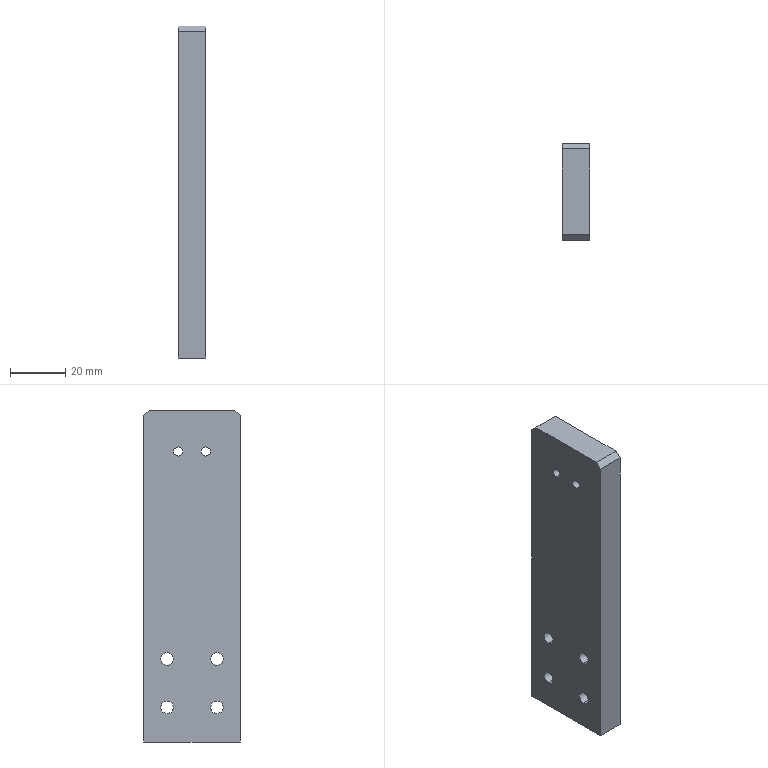Part | SolidWorks | features Chamfer 1, Extrusion 1, HoleWzd 1, ICE 1, LPattern 1 | 1 solid | 20 faces | box 10 x 35 x 120 mm | volume 41153 mm3 | cylinder 12 | plane 8 | commonest cylinder face diameters 4.5 x8 3.3 x4
STEP:
#1=CARTESIAN_POINT('',(10.,-9.,-27.75));
#2=VERTEX_POINT('',#1);
#3=CARTESIAN_POINT('',(10.,-9.,-32.25));
#4=VERTEX_POINT('',#3);
#5=CARTESIAN_POINT('',(10.,-9.,-30.));
#6=DIRECTION('',(1.,0.,0.));
#7=DIRECTION('',(0.,0.,-1.));
#8=AXIS2_PLACEMENT_3D('',#5,#6,#7);
#9=CIRCLE('',#8,2.25);
#10=EDGE_CURVE('',#2,#4,#9,.T.);
#11=ORIENTED_EDGE('',*,*,#10,.T.);
#12=CARTESIAN_POINT('',(0.,-9.,-32.25));
#13=VERTEX_POINT('',#12);
#14=CARTESIAN_POINT('',(28.,-9.,-32.25));
#15=DIRECTION('',(-1.,0.,0.));
#16=VECTOR('',#15,1000.);
#17=LINE('',#14,#16);
#18=EDGE_CURVE('',#4,#13,#17,.T.);
#19=ORIENTED_EDGE('',*,*,#18,.T.);
#20=CARTESIAN_POINT('',(0.,-9.,-27.75));
#21=VERTEX_POINT('',#20);
#22=CARTESIAN_POINT('',(0.,-9.,-30.));
#23=DIRECTION('',(-1.,0.,0.));
#24=DIRECTION('',(0.,0.,-1.));
#25=AXIS2_PLACEMENT_3D('',#22,#23,#24);
#26=CIRCLE('',#25,2.25);
#27=EDGE_CURVE('',#13,#21,#26,.T.);
#28=ORIENTED_EDGE('',*,*,#27,.T.);
#29=CARTESIAN_POINT('',(28.,-9.,-27.75));
#30=DIRECTION('',(-1.,0.,0.));
#31=VECTOR('',#30,1000.);
#32=LINE('',#29,#31);
#33=EDGE_CURVE('',#2,#21,#32,.T.);
#34=ORIENTED_EDGE('',*,*,#33,.F.);
#35=EDGE_LOOP('',(#11,#19,#28,#34));
#36=FACE_OUTER_BOUND('',#35,.T.);
#37=CARTESIAN_POINT('',(28.,-9.,-30.));
#38=DIRECTION('',(-1.,0.,0.));
#39=DIRECTION('',(0.,0.,1.));
#40=AXIS2_PLACEMENT_3D('',#37,#38,#39);
#41=CYLINDRICAL_SURFACE('',#40,2.25);
#42=ADVANCED_FACE('',(#36),#41,.F.);
#43=CARTESIAN_POINT('',(10.,9.,-27.75));
#44=VERTEX_POINT('',#43);
#45=CARTESIAN_POINT('',(10.,9.,-32.25));
#46=VERTEX_POINT('',#45);
#47=CARTESIAN_POINT('',(10.,9.,-30.));
#48=DIRECTION('',(1.,0.,0.));
#49=DIRECTION('',(0.,0.,-1.));
#50=AXIS2_PLACEMENT_3D('',#47,#48,#49);
#51=CIRCLE('',#50,2.25);
#52=EDGE_CURVE('',#44,#46,#51,.T.);
#53=ORIENTED_EDGE('',*,*,#52,.T.);
#54=CARTESIAN_POINT('',(0.,9.,-32.25));
#55=VERTEX_POINT('',#54);
#56=CARTESIAN_POINT('',(28.,9.,-32.25));
#57=DIRECTION('',(-1.,0.,0.));
#58=VECTOR('',#57,1000.);
#59=LINE('',#56,#58);
#60=EDGE_CURVE('',#46,#55,#59,.T.);
#61=ORIENTED_EDGE('',*,*,#60,.T.);
#62=CARTESIAN_POINT('',(0.,9.,-27.75));
#63=VERTEX_POINT('',#62);
#64=CARTESIAN_POINT('',(0.,9.,-30.));
#65=DIRECTION('',(-1.,0.,0.));
#66=DIRECTION('',(0.,0.,1.));
#67=AXIS2_PLACEMENT_3D('',#64,#65,#66);
#68=CIRCLE('',#67,2.25);
#69=EDGE_CURVE('',#55,#63,#68,.T.);
#70=ORIENTED_EDGE('',*,*,#69,.T.);
#71=CARTESIAN_POINT('',(28.,9.,-27.75));
#72=DIRECTION('',(-1.,0.,0.));
#73=VECTOR('',#72,1000.);
#74=LINE('',#71,#73);
#75=EDGE_CURVE('',#44,#63,#74,.T.);
#76=ORIENTED_EDGE('',*,*,#75,.F.);
#77=EDGE_LOOP('',(#53,#61,#70,#76));
#78=FACE_OUTER_BOUND('',#77,.T.);
#79=CARTESIAN_POINT('',(28.,9.,-30.));
#80=DIRECTION('',(-1.,0.,0.));
#81=DIRECTION('',(0.,0.,1.));
#82=AXIS2_PLACEMENT_3D('',#79,#80,#81);
#83=CYLINDRICAL_SURFACE('',#82,2.25);
#84=ADVANCED_FACE('',(#78),#83,.F.);
#85=CARTESIAN_POINT('',(10.,-9.,-45.25));
#86=VERTEX_POINT('',#85);
#87=CARTESIAN_POINT('',(10.,-9.,-49.75));
#88=VERTEX_POINT('',#87);
#89=CARTESIAN_POINT('',(10.,-9.,-47.5));
#90=DIRECTION('',(1.,0.,0.));
#91=DIRECTION('',(0.,0.,-1.));
#92=AXIS2_PLACEMENT_3D('',#89,#90,#91);
#93=CIRCLE('',#92,2.25);
#94=EDGE_CURVE('',#86,#88,#93,.T.);
#95=ORIENTED_EDGE('',*,*,#94,.T.);
#96=CARTESIAN_POINT('',(0.,-9.,-49.75));
#97=VERTEX_POINT('',#96);
#98=CARTESIAN_POINT('',(28.,-9.,-49.75));
#99=DIRECTION('',(-1.,0.,0.));
#100=VECTOR('',#99,1000.);
#101=LINE('',#98,#100);
#102=EDGE_CURVE('',#88,#97,#101,.T.);
#103=ORIENTED_EDGE('',*,*,#102,.T.);
#104=CARTESIAN_POINT('',(0.,-9.,-45.25));
#105=VERTEX_POINT('',#104);
#106=CARTESIAN_POINT('',(0.,-9.,-47.5));
#107=DIRECTION('',(-1.,0.,0.));
#108=DIRECTION('',(0.,0.,-1.));
#109=AXIS2_PLACEMENT_3D('',#106,#107,#108);
#110=CIRCLE('',#109,2.25);
#111=EDGE_CURVE('',#97,#105,#110,.T.);
#112=ORIENTED_EDGE('',*,*,#111,.T.);
#113=CARTESIAN_POINT('',(28.,-9.,-45.25));
#114=DIRECTION('',(-1.,0.,0.));
#115=VECTOR('',#114,1000.);
#116=LINE('',#113,#115);
#117=EDGE_CURVE('',#86,#105,#116,.T.);
#118=ORIENTED_EDGE('',*,*,#117,.F.);
#119=EDGE_LOOP('',(#95,#103,#112,#118));
#120=FACE_OUTER_BOUND('',#119,.T.);
#121=CARTESIAN_POINT('',(28.,-9.,-47.5));
#122=DIRECTION('',(-1.,0.,0.));
#123=DIRECTION('',(0.,0.,1.));
#124=AXIS2_PLACEMENT_3D('',#121,#122,#123);
#125=CYLINDRICAL_SURFACE('',#124,2.25);
#126=ADVANCED_FACE('',(#120),#125,.F.);
#127=CARTESIAN_POINT('',(10.,9.,-45.25));
#128=VERTEX_POINT('',#127);
#129=CARTESIAN_POINT('',(10.,9.,-49.75));
#130=VERTEX_POINT('',#129);
#131=CARTESIAN_POINT('',(10.,9.,-47.5));
#132=DIRECTION('',(1.,0.,0.));
#133=DIRECTION('',(0.,0.,-1.));
#134=AXIS2_PLACEMENT_3D('',#131,#132,#133);
#135=CIRCLE('',#134,2.25);
#136=EDGE_CURVE('',#128,#130,#135,.T.);
#137=ORIENTED_EDGE('',*,*,#136,.T.);
#138=CARTESIAN_POINT('',(0.,9.,-49.75));
#139=VERTEX_POINT('',#138);
#140=CARTESIAN_POINT('',(28.,9.,-49.75));
#141=DIRECTION('',(-1.,0.,0.));
#142=VECTOR('',#141,1000.);
#143=LINE('',#140,#142);
#144=EDGE_CURVE('',#130,#139,#143,.T.);
#145=ORIENTED_EDGE('',*,*,#144,.T.);
#146=CARTESIAN_POINT('',(0.,9.,-45.25));
#147=VERTEX_POINT('',#146);
#148=CARTESIAN_POINT('',(0.,9.,-47.5));
#149=DIRECTION('',(-1.,0.,0.));
#150=DIRECTION('',(0.,0.,1.));
#151=AXIS2_PLACEMENT_3D('',#148,#149,#150);
#152=CIRCLE('',#151,2.25);
#153=EDGE_CURVE('',#139,#147,#152,.T.);
#154=ORIENTED_EDGE('',*,*,#153,.T.);
#155=CARTESIAN_POINT('',(28.,9.,-45.25));
#156=DIRECTION('',(-1.,0.,0.));
#157=VECTOR('',#156,1000.);
#158=LINE('',#155,#157);
#159=EDGE_CURVE('',#128,#147,#158,.T.);
#160=ORIENTED_EDGE('',*,*,#159,.F.);
#161=EDGE_LOOP('',(#137,#145,#154,#160));
#162=FACE_OUTER_BOUND('',#161,.T.);
#163=CARTESIAN_POINT('',(28.,9.,-47.5));
#164=DIRECTION('',(-1.,0.,0.));
#165=DIRECTION('',(0.,0.,1.));
#166=AXIS2_PLACEMENT_3D('',#163,#164,#165);
#167=CYLINDRICAL_SURFACE('',#166,2.25);
#168=ADVANCED_FACE('',(#162),#167,.F.);
#169=CARTESIAN_POINT('',(10.,5.,43.35));
#170=VERTEX_POINT('',#169);
#171=CARTESIAN_POINT('',(10.,5.,46.65));
#172=VERTEX_POINT('',#171);
#173=CARTESIAN_POINT('',(10.,5.,45.));
#174=DIRECTION('',(-1.,0.,0.));
#175=DIRECTION('',(0.,0.,1.));
#176=AXIS2_PLACEMENT_3D('',#173,#174,#175);
#177=CIRCLE('',#176,1.65);
#178=EDGE_CURVE('',#170,#172,#177,.T.);
#179=ORIENTED_EDGE('',*,*,#178,.F.);
#180=CARTESIAN_POINT('',(0.,5.,43.35));
#181=VERTEX_POINT('',#180);
#182=CARTESIAN_POINT('',(0.,5.,43.35));
#183=DIRECTION('',(-1.,0.,0.));
#184=VECTOR('',#183,1000.);
#185=LINE('',#182,#184);
#186=EDGE_CURVE('',#170,#181,#185,.T.);
#187=ORIENTED_EDGE('',*,*,#186,.T.);
#188=CARTESIAN_POINT('',(0.,5.,46.65));
#189=VERTEX_POINT('',#188);
#190=CARTESIAN_POINT('',(0.,5.,45.));
#191=DIRECTION('',(-1.,0.,0.));
#192=DIRECTION('',(0.,0.,1.));
#193=AXIS2_PLACEMENT_3D('',#190,#191,#192);
#194=CIRCLE('',#193,1.65);
#195=EDGE_CURVE('',#181,#189,#194,.T.);
#196=ORIENTED_EDGE('',*,*,#195,.T.);
#197=CARTESIAN_POINT('',(0.,5.,46.65));
#198=DIRECTION('',(-1.,0.,0.));
#199=VECTOR('',#198,1000.);
#200=LINE('',#197,#199);
#201=EDGE_CURVE('',#172,#189,#200,.T.);
#202=ORIENTED_EDGE('',*,*,#201,.F.);
#203=EDGE_LOOP('',(#179,#187,#196,#202));
#204=FACE_OUTER_BOUND('',#203,.T.);
#205=CARTESIAN_POINT('',(0.,5.,45.));
#206=DIRECTION('',(-1.,0.,0.));
#207=DIRECTION('',(0.,0.,1.));
#208=AXIS2_PLACEMENT_3D('',#205,#206,#207);
#209=CYLINDRICAL_SURFACE('',#208,1.65);
#210=ADVANCED_FACE('',(#204),#209,.F.);
#211=CARTESIAN_POINT('',(10.,-5.,43.35));
#212=VERTEX_POINT('',#211);
#213=CARTESIAN_POINT('',(10.,-5.,46.65));
#214=VERTEX_POINT('',#213);
#215=CARTESIAN_POINT('',(10.,-5.,45.));
#216=DIRECTION('',(-1.,0.,0.));
#217=DIRECTION('',(0.,0.,1.));
#218=AXIS2_PLACEMENT_3D('',#215,#216,#217);
#219=CIRCLE('',#218,1.65);
#220=EDGE_CURVE('',#212,#214,#219,.T.);
#221=ORIENTED_EDGE('',*,*,#220,.F.);
#222=CARTESIAN_POINT('',(0.,-5.,43.35));
#223=VERTEX_POINT('',#222);
#224=CARTESIAN_POINT('',(0.,-5.,43.35));
#225=DIRECTION('',(-1.,0.,0.));
#226=VECTOR('',#225,1000.);
#227=LINE('',#224,#226);
#228=EDGE_CURVE('',#212,#223,#227,.T.);
#229=ORIENTED_EDGE('',*,*,#228,.T.);
#230=CARTESIAN_POINT('',(0.,-5.,46.65));
#231=VERTEX_POINT('',#230);
#232=CARTESIAN_POINT('',(0.,-5.,45.));
#233=DIRECTION('',(-1.,0.,0.));
#234=DIRECTION('',(0.,0.,1.));
#235=AXIS2_PLACEMENT_3D('',#232,#233,#234);
#236=CIRCLE('',#235,1.65);
#237=EDGE_CURVE('',#223,#231,#236,.T.);
#238=ORIENTED_EDGE('',*,*,#237,.T.);
#239=CARTESIAN_POINT('',(0.,-5.,46.65));
#240=DIRECTION('',(-1.,0.,0.));
#241=VECTOR('',#240,1000.);
#242=LINE('',#239,#241);
#243=EDGE_CURVE('',#214,#231,#242,.T.);
#244=ORIENTED_EDGE('',*,*,#243,.F.);
#245=EDGE_LOOP('',(#221,#229,#238,#244));
#246=FACE_OUTER_BOUND('',#245,.T.);
#247=CARTESIAN_POINT('',(0.,-5.,45.));
#248=DIRECTION('',(-1.,0.,0.));
#249=DIRECTION('',(0.,0.,1.));
#250=AXIS2_PLACEMENT_3D('',#247,#248,#249);
#251=CYLINDRICAL_SURFACE('',#250,1.65);
#252=ADVANCED_FACE('',(#246),#251,.F.);
#253=CARTESIAN_POINT('',(0.,-9.,-30.));
#254=DIRECTION('',(-1.,0.,0.));
#255=DIRECTION('',(0.,0.,-1.));
#256=AXIS2_PLACEMENT_3D('',#253,#254,#255);
#257=CIRCLE('',#256,2.25);
#258=EDGE_CURVE('',#21,#13,#257,.T.);
#259=ORIENTED_EDGE('',*,*,#258,.F.);
#260=ORIENTED_EDGE('',*,*,#27,.F.);
#261=EDGE_LOOP('',(#259,#260));
#262=FACE_BOUND('',#261,.T.);
#263=CARTESIAN_POINT('',(0.,9.,-30.));
#264=DIRECTION('',(-1.,0.,0.));
#265=DIRECTION('',(0.,0.,1.));
#266=AXIS2_PLACEMENT_3D('',#263,#264,#265);
#267=CIRCLE('',#266,2.25);
#268=EDGE_CURVE('',#63,#55,#267,.T.);
#269=ORIENTED_EDGE('',*,*,#268,.F.);
#270=ORIENTED_EDGE('',*,*,#69,.F.);
#271=EDGE_LOOP('',(#269,#270));
#272=FACE_BOUND('',#271,.T.);
#273=CARTESIAN_POINT('',(0.,-9.,-47.5));
#274=DIRECTION('',(-1.,0.,0.));
#275=DIRECTION('',(0.,0.,-1.));
#276=AXIS2_PLACEMENT_3D('',#273,#274,#275);
#277=CIRCLE('',#276,2.25);
#278=EDGE_CURVE('',#105,#97,#277,.T.);
#279=ORIENTED_EDGE('',*,*,#278,.F.);
#280=ORIENTED_EDGE('',*,*,#111,.F.);
#281=EDGE_LOOP('',(#279,#280));
#282=FACE_BOUND('',#281,.T.);
#283=CARTESIAN_POINT('',(0.,9.,-47.5));
#284=DIRECTION('',(-1.,0.,0.));
#285=DIRECTION('',(0.,0.,1.));
#286=AXIS2_PLACEMENT_3D('',#283,#284,#285);
#287=CIRCLE('',#286,2.25);
#288=EDGE_CURVE('',#147,#139,#287,.T.);
#289=ORIENTED_EDGE('',*,*,#288,.F.);
#290=ORIENTED_EDGE('',*,*,#153,.F.);
#291=EDGE_LOOP('',(#289,#290));
#292=FACE_BOUND('',#291,.T.);
#293=CARTESIAN_POINT('',(0.,-5.,45.));
#294=DIRECTION('',(-1.,0.,0.));
#295=DIRECTION('',(0.,0.,1.));
#296=AXIS2_PLACEMENT_3D('',#293,#294,#295);
#297=CIRCLE('',#296,1.65);
#298=EDGE_CURVE('',#231,#223,#297,.T.);
#299=ORIENTED_EDGE('',*,*,#298,.F.);
#300=ORIENTED_EDGE('',*,*,#237,.F.);
#301=EDGE_LOOP('',(#299,#300));
#302=FACE_BOUND('',#301,.T.);
#303=CARTESIAN_POINT('',(0.,-17.5,58.));
#304=VERTEX_POINT('',#303);
#305=CARTESIAN_POINT('',(0.,-17.5,-60.));
#306=VERTEX_POINT('',#305);
#307=CARTESIAN_POINT('',(0.,-17.5,60.));
#308=DIRECTION('',(0.,0.,-1.));
#309=VECTOR('',#308,1000.);
#310=LINE('',#307,#309);
#311=EDGE_CURVE('',#304,#306,#310,.T.);
#312=ORIENTED_EDGE('',*,*,#311,.F.);
#313=CARTESIAN_POINT('',(0.,-15.5,60.));
#314=VERTEX_POINT('',#313);
#315=CARTESIAN_POINT('',(0.,-17.5,58.));
#316=DIRECTION('',(0.,0.7071,0.7071));
#317=VECTOR('',#316,1000.);
#318=LINE('',#315,#317);
#319=EDGE_CURVE('',#304,#314,#318,.T.);
#320=ORIENTED_EDGE('',*,*,#319,.T.);
#321=CARTESIAN_POINT('',(0.,15.5,60.));
#322=VERTEX_POINT('',#321);
#323=CARTESIAN_POINT('',(0.,17.5,60.));
#324=DIRECTION('',(0.,-1.,0.));
#325=VECTOR('',#324,1000.);
#326=LINE('',#323,#325);
#327=EDGE_CURVE('',#322,#314,#326,.T.);
#328=ORIENTED_EDGE('',*,*,#327,.F.);
#329=CARTESIAN_POINT('',(0.,17.5,58.));
#330=VERTEX_POINT('',#329);
#331=CARTESIAN_POINT('',(0.,15.5,60.));
#332=DIRECTION('',(0.,0.7071,-0.7071));
#333=VECTOR('',#332,1000.);
#334=LINE('',#331,#333);
#335=EDGE_CURVE('',#322,#330,#334,.T.);
#336=ORIENTED_EDGE('',*,*,#335,.T.);
#337=CARTESIAN_POINT('',(0.,17.5,-60.));
#338=VERTEX_POINT('',#337);
#339=CARTESIAN_POINT('',(0.,17.5,60.));
#340=DIRECTION('',(0.,0.,1.));
#341=VECTOR('',#340,1000.);
#342=LINE('',#339,#341);
#343=EDGE_CURVE('',#338,#330,#342,.T.);
#344=ORIENTED_EDGE('',*,*,#343,.F.);
#345=CARTESIAN_POINT('',(0.,17.5,-60.));
#346=DIRECTION('',(0.,1.,0.));
#347=VECTOR('',#346,1000.);
#348=LINE('',#345,#347);
#349=EDGE_CURVE('',#306,#338,#348,.T.);
#350=ORIENTED_EDGE('',*,*,#349,.F.);
#351=EDGE_LOOP('',(#312,#320,#328,#336,#344,#350));
#352=FACE_OUTER_BOUND('',#351,.T.);
#353=CARTESIAN_POINT('',(0.,5.,45.));
#354=DIRECTION('',(-1.,0.,0.));
#355=DIRECTION('',(0.,0.,1.));
#356=AXIS2_PLACEMENT_3D('',#353,#354,#355);
#357=CIRCLE('',#356,1.65);
#358=EDGE_CURVE('',#189,#181,#357,.T.);
#359=ORIENTED_EDGE('',*,*,#358,.F.);
#360=ORIENTED_EDGE('',*,*,#195,.F.);
#361=EDGE_LOOP('',(#359,#360));
#362=FACE_BOUND('',#361,.T.);
#363=CARTESIAN_POINT('',(0.,0.,0.));
#364=DIRECTION('',(1.,0.,0.));
#365=DIRECTION('',(0.,0.,-1.));
#366=AXIS2_PLACEMENT_3D('',#363,#364,#365);
#367=PLANE('',#366);
#368=ADVANCED_FACE('',(#262,#272,#282,#292,#302,#352,#362),#367,.F.);
#369=ORIENTED_EDGE('',*,*,#349,.T.);
#370=CARTESIAN_POINT('',(10.,17.5,-60.));
#371=VERTEX_POINT('',#370);
#372=CARTESIAN_POINT('',(10.,17.5,-60.));
#373=DIRECTION('',(-1.,0.,0.));
#374=VECTOR('',#373,1000.);
#375=LINE('',#372,#374);
#376=EDGE_CURVE('',#371,#338,#375,.T.);
#377=ORIENTED_EDGE('',*,*,#376,.F.);
#378=CARTESIAN_POINT('',(10.,-17.5,-60.));
#379=VERTEX_POINT('',#378);
#380=CARTESIAN_POINT('',(10.,17.5,-60.));
#381=DIRECTION('',(0.,1.,0.));
#382=VECTOR('',#381,1000.);
#383=LINE('',#380,#382);
#384=EDGE_CURVE('',#379,#371,#383,.T.);
#385=ORIENTED_EDGE('',*,*,#384,.F.);
#386=CARTESIAN_POINT('',(10.,-17.5,-60.));
#387=DIRECTION('',(-1.,0.,0.));
#388=VECTOR('',#387,1000.);
#389=LINE('',#386,#388);
#390=EDGE_CURVE('',#379,#306,#389,.T.);
#391=ORIENTED_EDGE('',*,*,#390,.T.);
#392=EDGE_LOOP('',(#369,#377,#385,#391));
#393=FACE_OUTER_BOUND('',#392,.T.);
#394=CARTESIAN_POINT('',(10.,17.5,-60.));
#395=DIRECTION('',(0.,0.,1.));
#396=DIRECTION('',(0.,-1.,0.));
#397=AXIS2_PLACEMENT_3D('',#394,#395,#396);
#398=PLANE('',#397);
#399=ADVANCED_FACE('',(#393),#398,.F.);
#400=ORIENTED_EDGE('',*,*,#343,.T.);
#401=CARTESIAN_POINT('',(10.,17.5,58.));
#402=VERTEX_POINT('',#401);
#403=CARTESIAN_POINT('',(10.,17.5,58.));
#404=DIRECTION('',(1.,0.,0.));
#405=VECTOR('',#404,1000.);
#406=LINE('',#403,#405);
#407=EDGE_CURVE('',#330,#402,#406,.T.);
#408=ORIENTED_EDGE('',*,*,#407,.T.);
#409=CARTESIAN_POINT('',(10.,17.5,60.));
#410=DIRECTION('',(0.,0.,1.));
#411=VECTOR('',#410,1000.);
#412=LINE('',#409,#411);
#413=EDGE_CURVE('',#371,#402,#412,.T.);
#414=ORIENTED_EDGE('',*,*,#413,.F.);
#415=ORIENTED_EDGE('',*,*,#376,.T.);
#416=EDGE_LOOP('',(#400,#408,#414,#415));
#417=FACE_OUTER_BOUND('',#416,.T.);
#418=CARTESIAN_POINT('',(10.,17.5,60.));
#419=DIRECTION('',(0.,-1.,0.));
#420=DIRECTION('',(0.,0.,-1.));
#421=AXIS2_PLACEMENT_3D('',#418,#419,#420);
#422=PLANE('',#421);
#423=ADVANCED_FACE('',(#417),#422,.F.);
#424=ORIENTED_EDGE('',*,*,#327,.T.);
#425=CARTESIAN_POINT('',(10.,-15.5,60.));
#426=VERTEX_POINT('',#425);
#427=CARTESIAN_POINT('',(10.,-15.5,60.));
#428=DIRECTION('',(1.,0.,0.));
#429=VECTOR('',#428,1000.);
#430=LINE('',#427,#429);
#431=EDGE_CURVE('',#314,#426,#430,.T.);
#432=ORIENTED_EDGE('',*,*,#431,.T.);
#433=CARTESIAN_POINT('',(10.,15.5,60.));
#434=VERTEX_POINT('',#433);
#435=CARTESIAN_POINT('',(10.,17.5,60.));
#436=DIRECTION('',(0.,-1.,0.));
#437=VECTOR('',#436,1000.);
#438=LINE('',#435,#437);
#439=EDGE_CURVE('',#434,#426,#438,.T.);
#440=ORIENTED_EDGE('',*,*,#439,.F.);
#441=CARTESIAN_POINT('',(10.,15.5,60.));
#442=DIRECTION('',(-1.,0.,0.));
#443=VECTOR('',#442,1000.);
#444=LINE('',#441,#443);
#445=EDGE_CURVE('',#434,#322,#444,.T.);
#446=ORIENTED_EDGE('',*,*,#445,.T.);
#447=EDGE_LOOP('',(#424,#432,#440,#446));
#448=FACE_OUTER_BOUND('',#447,.T.);
#449=CARTESIAN_POINT('',(10.,17.5,60.));
#450=DIRECTION('',(0.,0.,-1.));
#451=DIRECTION('',(-1.,0.,0.));
#452=AXIS2_PLACEMENT_3D('',#449,#450,#451);
#453=PLANE('',#452);
#454=ADVANCED_FACE('',(#448),#453,.F.);
#455=CARTESIAN_POINT('',(10.,-17.5,58.));
#456=VERTEX_POINT('',#455);
#457=CARTESIAN_POINT('',(10.,-17.5,60.));
#458=DIRECTION('',(0.,0.,-1.));
#459=VECTOR('',#458,1000.);
#460=LINE('',#457,#459);
#461=EDGE_CURVE('',#456,#379,#460,.T.);
#462=ORIENTED_EDGE('',*,*,#461,.F.);
#463=CARTESIAN_POINT('',(10.,-17.5,58.));
#464=DIRECTION('',(-1.,0.,0.));
#465=VECTOR('',#464,1000.);
#466=LINE('',#463,#465);
#467=EDGE_CURVE('',#456,#304,#466,.T.);
#468=ORIENTED_EDGE('',*,*,#467,.T.);
#469=ORIENTED_EDGE('',*,*,#311,.T.);
#470=ORIENTED_EDGE('',*,*,#390,.F.);
#471=EDGE_LOOP('',(#462,#468,#469,#470));
#472=FACE_OUTER_BOUND('',#471,.T.);
#473=CARTESIAN_POINT('',(10.,-17.5,60.));
#474=DIRECTION('',(0.,1.,0.));
#475=DIRECTION('',(0.,0.,1.));
#476=AXIS2_PLACEMENT_3D('',#473,#474,#475);
#477=PLANE('',#476);
#478=ADVANCED_FACE('',(#472),#477,.F.);
#479=ORIENTED_EDGE('',*,*,#10,.F.);
#480=CARTESIAN_POINT('',(10.,-9.,-30.));
#481=DIRECTION('',(1.,0.,0.));
#482=DIRECTION('',(0.,0.,-1.));
#483=AXIS2_PLACEMENT_3D('',#480,#481,#482);
#484=CIRCLE('',#483,2.25);
#485=EDGE_CURVE('',#4,#2,#484,.T.);
#486=ORIENTED_EDGE('',*,*,#485,.F.);
#487=EDGE_LOOP('',(#479,#486));
#488=FACE_BOUND('',#487,.T.);
#489=ORIENTED_EDGE('',*,*,#52,.F.);
#490=CARTESIAN_POINT('',(10.,9.,-30.));
#491=DIRECTION('',(1.,0.,0.));
#492=DIRECTION('',(0.,0.,-1.));
#493=AXIS2_PLACEMENT_3D('',#490,#491,#492);
#494=CIRCLE('',#493,2.25);
#495=EDGE_CURVE('',#46,#44,#494,.T.);
#496=ORIENTED_EDGE('',*,*,#495,.F.);
#497=EDGE_LOOP('',(#489,#496));
#498=FACE_BOUND('',#497,.T.);
#499=ORIENTED_EDGE('',*,*,#94,.F.);
#500=CARTESIAN_POINT('',(10.,-9.,-47.5));
#501=DIRECTION('',(1.,0.,0.));
#502=DIRECTION('',(0.,0.,-1.));
#503=AXIS2_PLACEMENT_3D('',#500,#501,#502);
#504=CIRCLE('',#503,2.25);
#505=EDGE_CURVE('',#88,#86,#504,.T.);
#506=ORIENTED_EDGE('',*,*,#505,.F.);
#507=EDGE_LOOP('',(#499,#506));
#508=FACE_BOUND('',#507,.T.);
#509=ORIENTED_EDGE('',*,*,#136,.F.);
#510=CARTESIAN_POINT('',(10.,9.,-47.5));
#511=DIRECTION('',(1.,0.,0.));
#512=DIRECTION('',(0.,0.,-1.));
#513=AXIS2_PLACEMENT_3D('',#510,#511,#512);
#514=CIRCLE('',#513,2.25);
#515=EDGE_CURVE('',#130,#128,#514,.T.);
#516=ORIENTED_EDGE('',*,*,#515,.F.);
#517=EDGE_LOOP('',(#509,#516));
#518=FACE_BOUND('',#517,.T.);
#519=CARTESIAN_POINT('',(10.,5.,45.));
#520=DIRECTION('',(-1.,0.,0.));
#521=DIRECTION('',(0.,0.,1.));
#522=AXIS2_PLACEMENT_3D('',#519,#520,#521);
#523=CIRCLE('',#522,1.65);
#524=EDGE_CURVE('',#172,#170,#523,.T.);
#525=ORIENTED_EDGE('',*,*,#524,.T.);
#526=ORIENTED_EDGE('',*,*,#178,.T.);
#527=EDGE_LOOP('',(#525,#526));
#528=FACE_BOUND('',#527,.T.);
#529=CARTESIAN_POINT('',(10.,-5.,45.));
#530=DIRECTION('',(-1.,0.,0.));
#531=DIRECTION('',(0.,0.,1.));
#532=AXIS2_PLACEMENT_3D('',#529,#530,#531);
#533=CIRCLE('',#532,1.65);
#534=EDGE_CURVE('',#214,#212,#533,.T.);
#535=ORIENTED_EDGE('',*,*,#534,.T.);
#536=ORIENTED_EDGE('',*,*,#220,.T.);
#537=EDGE_LOOP('',(#535,#536));
#538=FACE_BOUND('',#537,.T.);
#539=ORIENTED_EDGE('',*,*,#439,.T.);
#540=CARTESIAN_POINT('',(10.,-37.75,37.75));
#541=DIRECTION('',(0.,-0.7071,-0.7071));
#542=VECTOR('',#541,1000.);
#543=LINE('',#540,#542);
#544=EDGE_CURVE('',#426,#456,#543,.T.);
#545=ORIENTED_EDGE('',*,*,#544,.T.);
#546=ORIENTED_EDGE('',*,*,#461,.T.);
#547=ORIENTED_EDGE('',*,*,#384,.T.);
#548=ORIENTED_EDGE('',*,*,#413,.T.);
#549=CARTESIAN_POINT('',(10.,37.75,37.75));
#550=DIRECTION('',(0.,-0.7071,0.7071));
#551=VECTOR('',#550,1000.);
#552=LINE('',#549,#551);
#553=EDGE_CURVE('',#402,#434,#552,.T.);
#554=ORIENTED_EDGE('',*,*,#553,.T.);
#555=EDGE_LOOP('',(#539,#545,#546,#547,#548,#554));
#556=FACE_OUTER_BOUND('',#555,.T.);
#557=CARTESIAN_POINT('',(10.,0.,0.));
#558=DIRECTION('',(1.,0.,0.));
#559=DIRECTION('',(0.,0.,-1.));
#560=AXIS2_PLACEMENT_3D('',#557,#558,#559);
#561=PLANE('',#560);
#562=ADVANCED_FACE('',(#488,#498,#508,#518,#528,#538,#556),#561,.T.);
#563=ORIENTED_EDGE('',*,*,#228,.F.);
#564=ORIENTED_EDGE('',*,*,#534,.F.);
#565=ORIENTED_EDGE('',*,*,#243,.T.);
#566=ORIENTED_EDGE('',*,*,#298,.T.);
#567=EDGE_LOOP('',(#563,#564,#565,#566));
#568=FACE_OUTER_BOUND('',#567,.T.);
#569=CARTESIAN_POINT('',(0.,-5.,45.));
#570=DIRECTION('',(-1.,0.,0.));
#571=DIRECTION('',(0.,0.,1.));
#572=AXIS2_PLACEMENT_3D('',#569,#570,#571);
#573=CYLINDRICAL_SURFACE('',#572,1.65);
#574=ADVANCED_FACE('',(#568),#573,.F.);
#575=ORIENTED_EDGE('',*,*,#186,.F.);
#576=ORIENTED_EDGE('',*,*,#524,.F.);
#577=ORIENTED_EDGE('',*,*,#201,.T.);
#578=ORIENTED_EDGE('',*,*,#358,.T.);
#579=EDGE_LOOP('',(#575,#576,#577,#578));
#580=FACE_OUTER_BOUND('',#579,.T.);
#581=CARTESIAN_POINT('',(0.,5.,45.));
#582=DIRECTION('',(-1.,0.,0.));
#583=DIRECTION('',(0.,0.,1.));
#584=AXIS2_PLACEMENT_3D('',#581,#582,#583);
#585=CYLINDRICAL_SURFACE('',#584,1.65);
#586=ADVANCED_FACE('',(#580),#585,.F.);
#587=ORIENTED_EDGE('',*,*,#144,.F.);
#588=ORIENTED_EDGE('',*,*,#515,.T.);
#589=ORIENTED_EDGE('',*,*,#159,.T.);
#590=ORIENTED_EDGE('',*,*,#288,.T.);
#591=EDGE_LOOP('',(#587,#588,#589,#590));
#592=FACE_OUTER_BOUND('',#591,.T.);
#593=CARTESIAN_POINT('',(28.,9.,-47.5));
#594=DIRECTION('',(-1.,0.,0.));
#595=DIRECTION('',(0.,0.,1.));
#596=AXIS2_PLACEMENT_3D('',#593,#594,#595);
#597=CYLINDRICAL_SURFACE('',#596,2.25);
#598=ADVANCED_FACE('',(#592),#597,.F.);
#599=ORIENTED_EDGE('',*,*,#102,.F.);
#600=ORIENTED_EDGE('',*,*,#505,.T.);
#601=ORIENTED_EDGE('',*,*,#117,.T.);
#602=ORIENTED_EDGE('',*,*,#278,.T.);
#603=EDGE_LOOP('',(#599,#600,#601,#602));
#604=FACE_OUTER_BOUND('',#603,.T.);
#605=CARTESIAN_POINT('',(28.,-9.,-47.5));
#606=DIRECTION('',(-1.,0.,0.));
#607=DIRECTION('',(0.,0.,1.));
#608=AXIS2_PLACEMENT_3D('',#605,#606,#607);
#609=CYLINDRICAL_SURFACE('',#608,2.25);
#610=ADVANCED_FACE('',(#604),#609,.F.);
#611=ORIENTED_EDGE('',*,*,#544,.F.);
#612=ORIENTED_EDGE('',*,*,#431,.F.);
#613=ORIENTED_EDGE('',*,*,#319,.F.);
#614=ORIENTED_EDGE('',*,*,#467,.F.);
#615=EDGE_LOOP('',(#611,#612,#613,#614));
#616=FACE_OUTER_BOUND('',#615,.T.);
#617=CARTESIAN_POINT('',(10.,-17.5,58.));
#618=DIRECTION('',(0.,0.7071,-0.7071));
#619=DIRECTION('',(-1.,0.,0.));
#620=AXIS2_PLACEMENT_3D('',#617,#618,#619);
#621=PLANE('',#620);
#622=ADVANCED_FACE('',(#616),#621,.F.);
#623=ORIENTED_EDGE('',*,*,#553,.F.);
#624=ORIENTED_EDGE('',*,*,#407,.F.);
#625=ORIENTED_EDGE('',*,*,#335,.F.);
#626=ORIENTED_EDGE('',*,*,#445,.F.);
#627=EDGE_LOOP('',(#623,#624,#625,#626));
#628=FACE_OUTER_BOUND('',#627,.T.);
#629=CARTESIAN_POINT('',(10.,15.5,60.));
#630=DIRECTION('',(0.,-0.7071,-0.7071));
#631=DIRECTION('',(-1.,0.,0.));
#632=AXIS2_PLACEMENT_3D('',#629,#630,#631);
#633=PLANE('',#632);
#634=ADVANCED_FACE('',(#628),#633,.F.);
#635=ORIENTED_EDGE('',*,*,#60,.F.);
#636=ORIENTED_EDGE('',*,*,#495,.T.);
#637=ORIENTED_EDGE('',*,*,#75,.T.);
#638=ORIENTED_EDGE('',*,*,#268,.T.);
#639=EDGE_LOOP('',(#635,#636,#637,#638));
#640=FACE_OUTER_BOUND('',#639,.T.);
#641=CARTESIAN_POINT('',(28.,9.,-30.));
#642=DIRECTION('',(-1.,0.,0.));
#643=DIRECTION('',(0.,0.,1.));
#644=AXIS2_PLACEMENT_3D('',#641,#642,#643);
#645=CYLINDRICAL_SURFACE('',#644,2.25);
#646=ADVANCED_FACE('',(#640),#645,.F.);
#647=ORIENTED_EDGE('',*,*,#18,.F.);
#648=ORIENTED_EDGE('',*,*,#485,.T.);
#649=ORIENTED_EDGE('',*,*,#33,.T.);
#650=ORIENTED_EDGE('',*,*,#258,.T.);
#651=EDGE_LOOP('',(#647,#648,#649,#650));
#652=FACE_OUTER_BOUND('',#651,.T.);
#653=CARTESIAN_POINT('',(28.,-9.,-30.));
#654=DIRECTION('',(-1.,0.,0.));
#655=DIRECTION('',(0.,0.,1.));
#656=AXIS2_PLACEMENT_3D('',#653,#654,#655);
#657=CYLINDRICAL_SURFACE('',#656,2.25);
#658=ADVANCED_FACE('',(#652),#657,.F.);
#659=CLOSED_SHELL('',(#42,#84,#126,#168,#210,#252,#368,#399,#423,#454,#478,#562,#574,#586,#598,#610,#622,#634,#646,#658));
#660=MANIFOLD_SOLID_BREP('',#659);
#661=CARTESIAN_POINT('',(0.,0.,0.));
#662=DIRECTION('',(0.,0.,1.));
#663=DIRECTION('',(1.,0.,0.));
#664=AXIS2_PLACEMENT_3D('',#661,#662,#663);
#665=(LENGTH_UNIT()NAMED_UNIT(*)SI_UNIT(.MILLI.,.METRE.));
#666=UNCERTAINTY_MEASURE_WITH_UNIT(LENGTH_MEASURE(0.00001),#665,'','');
#667=(NAMED_UNIT(*)PLANE_ANGLE_UNIT()SI_UNIT($,.RADIAN.));
#668=(NAMED_UNIT(*)SI_UNIT($,.STERADIAN.)SOLID_ANGLE_UNIT());
#669=(GEOMETRIC_REPRESENTATION_CONTEXT(3)GLOBAL_UNCERTAINTY_ASSIGNED_CONTEXT((#666))GLOBAL_UNIT_ASSIGNED_CONTEXT((#665,#667,#668))REPRESENTATION_CONTEXT('',''));
#670=ADVANCED_BREP_SHAPE_REPRESENTATION('',(#660,#664),#669);